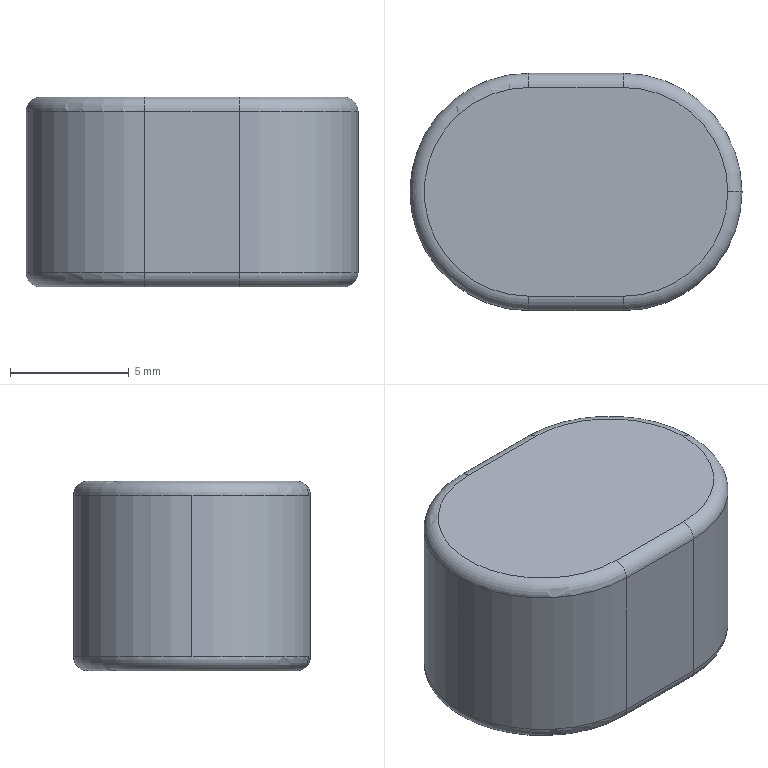Part | SolidWorks | features Extrusion 1, Fillet 1 | 1 solid | 17 faces | box 14 x 10 x 8 mm | volume 942.358 mm3 | cylinder 7 | torus 6 | plane 4 | commonest cylinder face diameters 1.2 x4 10 x3
STEP:
#1=CARTESIAN_POINT('',(6.4,0.,0.));
#2=VERTEX_POINT('',#1);
#3=CARTESIAN_POINT('',(2.,-4.4,0.));
#4=VERTEX_POINT('',#3);
#5=CARTESIAN_POINT('',(2.,0.,0.));
#6=DIRECTION('',(0.,0.,-1.));
#7=DIRECTION('',(1.,0.,0.));
#8=AXIS2_PLACEMENT_3D('',#5,#6,#7);
#9=CIRCLE('',#8,4.4);
#10=EDGE_CURVE('',#2,#4,#9,.T.);
#11=ORIENTED_EDGE('',*,*,#10,.F.);
#12=CARTESIAN_POINT('',(7.,0.,0.6));
#13=VERTEX_POINT('',#12);
#14=CARTESIAN_POINT('',(6.4,0.,0.6));
#15=DIRECTION('',(0.,-1.,0.));
#16=DIRECTION('',(0.,0.,-1.));
#17=AXIS2_PLACEMENT_3D('',#14,#15,#16);
#18=CIRCLE('',#17,0.6);
#19=EDGE_CURVE('',#2,#13,#18,.T.);
#20=ORIENTED_EDGE('',*,*,#19,.T.);
#21=CARTESIAN_POINT('',(2.,-5.,0.6));
#22=VERTEX_POINT('',#21);
#23=CARTESIAN_POINT('',(2.,0.,0.6));
#24=DIRECTION('',(0.,0.,1.));
#25=DIRECTION('',(1.,0.,0.));
#26=AXIS2_PLACEMENT_3D('',#23,#24,#25);
#27=CIRCLE('',#26,5.);
#28=EDGE_CURVE('',#22,#13,#27,.T.);
#29=ORIENTED_EDGE('',*,*,#28,.F.);
#30=CARTESIAN_POINT('',(2.,-4.4,0.6));
#31=DIRECTION('',(1.,0.,0.));
#32=DIRECTION('',(0.,0.,-1.));
#33=AXIS2_PLACEMENT_3D('',#30,#31,#32);
#34=CIRCLE('',#33,0.6);
#35=EDGE_CURVE('',#22,#4,#34,.T.);
#36=ORIENTED_EDGE('',*,*,#35,.T.);
#37=EDGE_LOOP('',(#11,#20,#29,#36));
#38=FACE_OUTER_BOUND('',#37,.T.);
#39=CARTESIAN_POINT('',(2.,0.,0.6));
#40=DIRECTION('',(0.,0.,1.));
#41=DIRECTION('',(1.,0.,0.));
#42=AXIS2_PLACEMENT_3D('',#39,#40,#41);
#43=TOROIDAL_SURFACE('',#42,4.4,0.6);
#44=ADVANCED_FACE('',(#38),#43,.T.);
#45=CARTESIAN_POINT('',(7.,0.,7.4));
#46=VERTEX_POINT('',#45);
#47=CARTESIAN_POINT('',(2.,-5.,7.4));
#48=VERTEX_POINT('',#47);
#49=CARTESIAN_POINT('',(2.,0.,7.4));
#50=DIRECTION('',(0.,0.,-1.));
#51=DIRECTION('',(1.,0.,0.));
#52=AXIS2_PLACEMENT_3D('',#49,#50,#51);
#53=CIRCLE('',#52,5.);
#54=EDGE_CURVE('',#46,#48,#53,.T.);
#55=ORIENTED_EDGE('',*,*,#54,.F.);
#56=CARTESIAN_POINT('',(6.4,0.,8.));
#57=VERTEX_POINT('',#56);
#58=CARTESIAN_POINT('',(6.4,0.,7.4));
#59=DIRECTION('',(0.,-1.,0.));
#60=DIRECTION('',(0.,0.,-1.));
#61=AXIS2_PLACEMENT_3D('',#58,#59,#60);
#62=CIRCLE('',#61,0.6);
#63=EDGE_CURVE('',#46,#57,#62,.T.);
#64=ORIENTED_EDGE('',*,*,#63,.T.);
#65=CARTESIAN_POINT('',(2.,-4.4,8.));
#66=VERTEX_POINT('',#65);
#67=CARTESIAN_POINT('',(2.,0.,8.));
#68=DIRECTION('',(0.,0.,1.));
#69=DIRECTION('',(1.,0.,0.));
#70=AXIS2_PLACEMENT_3D('',#67,#68,#69);
#71=CIRCLE('',#70,4.4);
#72=EDGE_CURVE('',#66,#57,#71,.T.);
#73=ORIENTED_EDGE('',*,*,#72,.F.);
#74=CARTESIAN_POINT('',(2.,-4.4,7.4));
#75=DIRECTION('',(1.,0.,0.));
#76=DIRECTION('',(0.,0.,-1.));
#77=AXIS2_PLACEMENT_3D('',#74,#75,#76);
#78=CIRCLE('',#77,0.6);
#79=EDGE_CURVE('',#66,#48,#78,.T.);
#80=ORIENTED_EDGE('',*,*,#79,.T.);
#81=EDGE_LOOP('',(#55,#64,#73,#80));
#82=FACE_OUTER_BOUND('',#81,.T.);
#83=CARTESIAN_POINT('',(2.,0.,7.4));
#84=DIRECTION('',(0.,0.,1.));
#85=DIRECTION('',(1.,0.,0.));
#86=AXIS2_PLACEMENT_3D('',#83,#84,#85);
#87=TOROIDAL_SURFACE('',#86,4.4,0.6);
#88=ADVANCED_FACE('',(#82),#87,.T.);
#89=CARTESIAN_POINT('',(-2.,-5.,7.4));
#90=VERTEX_POINT('',#89);
#91=CARTESIAN_POINT('',(-7.,0.,7.4));
#92=VERTEX_POINT('',#91);
#93=CARTESIAN_POINT('',(-2.,0.,7.4));
#94=DIRECTION('',(0.,0.,-1.));
#95=DIRECTION('',(1.,0.,0.));
#96=AXIS2_PLACEMENT_3D('',#93,#94,#95);
#97=CIRCLE('',#96,5.);
#98=EDGE_CURVE('',#90,#92,#97,.T.);
#99=ORIENTED_EDGE('',*,*,#98,.T.);
#100=CARTESIAN_POINT('',(-7.,0.,0.6));
#101=VERTEX_POINT('',#100);
#102=CARTESIAN_POINT('',(-7.,0.,8.));
#103=DIRECTION('',(0.,0.,-1.));
#104=VECTOR('',#103,1000.);
#105=LINE('',#102,#104);
#106=EDGE_CURVE('',#92,#101,#105,.T.);
#107=ORIENTED_EDGE('',*,*,#106,.T.);
#108=CARTESIAN_POINT('',(-2.,-5.,0.6));
#109=VERTEX_POINT('',#108);
#110=CARTESIAN_POINT('',(-2.,0.,0.6));
#111=DIRECTION('',(0.,0.,1.));
#112=DIRECTION('',(1.,0.,0.));
#113=AXIS2_PLACEMENT_3D('',#110,#111,#112);
#114=CIRCLE('',#113,5.);
#115=EDGE_CURVE('',#101,#109,#114,.T.);
#116=ORIENTED_EDGE('',*,*,#115,.T.);
#117=CARTESIAN_POINT('',(-2.,-5.,8.));
#118=DIRECTION('',(0.,0.,-1.));
#119=VECTOR('',#118,1000.);
#120=LINE('',#117,#119);
#121=EDGE_CURVE('',#90,#109,#120,.T.);
#122=ORIENTED_EDGE('',*,*,#121,.F.);
#123=EDGE_LOOP('',(#99,#107,#116,#122));
#124=FACE_OUTER_BOUND('',#123,.T.);
#125=CARTESIAN_POINT('',(-2.,0.,8.));
#126=DIRECTION('',(0.,0.,-1.));
#127=DIRECTION('',(-1.,0.,0.));
#128=AXIS2_PLACEMENT_3D('',#125,#126,#127);
#129=CYLINDRICAL_SURFACE('',#128,5.);
#130=ADVANCED_FACE('',(#124),#129,.T.);
#131=ORIENTED_EDGE('',*,*,#106,.F.);
#132=CARTESIAN_POINT('',(-2.,5.,7.4));
#133=VERTEX_POINT('',#132);
#134=CARTESIAN_POINT('',(-2.,0.,7.4));
#135=DIRECTION('',(0.,0.,-1.));
#136=DIRECTION('',(1.,0.,0.));
#137=AXIS2_PLACEMENT_3D('',#134,#135,#136);
#138=CIRCLE('',#137,5.);
#139=EDGE_CURVE('',#92,#133,#138,.T.);
#140=ORIENTED_EDGE('',*,*,#139,.T.);
#141=CARTESIAN_POINT('',(-2.,5.,0.6));
#142=VERTEX_POINT('',#141);
#143=CARTESIAN_POINT('',(-2.,5.,8.));
#144=DIRECTION('',(0.,0.,-1.));
#145=VECTOR('',#144,1000.);
#146=LINE('',#143,#145);
#147=EDGE_CURVE('',#133,#142,#146,.T.);
#148=ORIENTED_EDGE('',*,*,#147,.T.);
#149=CARTESIAN_POINT('',(-2.,0.,0.6));
#150=DIRECTION('',(0.,0.,1.));
#151=DIRECTION('',(1.,0.,0.));
#152=AXIS2_PLACEMENT_3D('',#149,#150,#151);
#153=CIRCLE('',#152,5.);
#154=EDGE_CURVE('',#142,#101,#153,.T.);
#155=ORIENTED_EDGE('',*,*,#154,.T.);
#156=EDGE_LOOP('',(#131,#140,#148,#155));
#157=FACE_OUTER_BOUND('',#156,.T.);
#158=CARTESIAN_POINT('',(-2.,0.,8.));
#159=DIRECTION('',(0.,0.,-1.));
#160=DIRECTION('',(-1.,0.,0.));
#161=AXIS2_PLACEMENT_3D('',#158,#159,#160);
#162=CYLINDRICAL_SURFACE('',#161,5.);
#163=ADVANCED_FACE('',(#157),#162,.T.);
#164=CARTESIAN_POINT('',(2.,-5.,8.));
#165=DIRECTION('',(0.,0.,-1.));
#166=VECTOR('',#165,1000.);
#167=LINE('',#164,#166);
#168=EDGE_CURVE('',#48,#22,#167,.T.);
#169=ORIENTED_EDGE('',*,*,#168,.F.);
#170=CARTESIAN_POINT('',(-2.,-5.,7.4));
#171=DIRECTION('',(-1.,0.,0.));
#172=VECTOR('',#171,1000.);
#173=LINE('',#170,#172);
#174=EDGE_CURVE('',#48,#90,#173,.T.);
#175=ORIENTED_EDGE('',*,*,#174,.T.);
#176=ORIENTED_EDGE('',*,*,#121,.T.);
#177=CARTESIAN_POINT('',(-2.,-5.,0.6));
#178=DIRECTION('',(1.,0.,0.));
#179=VECTOR('',#178,1000.);
#180=LINE('',#177,#179);
#181=EDGE_CURVE('',#109,#22,#180,.T.);
#182=ORIENTED_EDGE('',*,*,#181,.T.);
#183=EDGE_LOOP('',(#169,#175,#176,#182));
#184=FACE_OUTER_BOUND('',#183,.T.);
#185=CARTESIAN_POINT('',(-2.,-5.,8.));
#186=DIRECTION('',(0.,1.,0.));
#187=DIRECTION('',(-1.,0.,0.));
#188=AXIS2_PLACEMENT_3D('',#185,#186,#187);
#189=PLANE('',#188);
#190=ADVANCED_FACE('',(#184),#189,.F.);
#191=CARTESIAN_POINT('',(2.,5.,7.4));
#192=VERTEX_POINT('',#191);
#193=CARTESIAN_POINT('',(2.,5.,0.6));
#194=VERTEX_POINT('',#193);
#195=CARTESIAN_POINT('',(2.,5.,8.));
#196=DIRECTION('',(0.,0.,-1.));
#197=VECTOR('',#196,1000.);
#198=LINE('',#195,#197);
#199=EDGE_CURVE('',#192,#194,#198,.T.);
#200=ORIENTED_EDGE('',*,*,#199,.F.);
#201=CARTESIAN_POINT('',(2.,0.,7.4));
#202=DIRECTION('',(0.,0.,-1.));
#203=DIRECTION('',(1.,0.,0.));
#204=AXIS2_PLACEMENT_3D('',#201,#202,#203);
#205=CIRCLE('',#204,5.);
#206=EDGE_CURVE('',#192,#46,#205,.T.);
#207=ORIENTED_EDGE('',*,*,#206,.T.);
#208=ORIENTED_EDGE('',*,*,#54,.T.);
#209=ORIENTED_EDGE('',*,*,#168,.T.);
#210=ORIENTED_EDGE('',*,*,#28,.T.);
#211=CARTESIAN_POINT('',(2.,0.,0.6));
#212=DIRECTION('',(0.,0.,1.));
#213=DIRECTION('',(1.,0.,0.));
#214=AXIS2_PLACEMENT_3D('',#211,#212,#213);
#215=CIRCLE('',#214,5.);
#216=EDGE_CURVE('',#13,#194,#215,.T.);
#217=ORIENTED_EDGE('',*,*,#216,.T.);
#218=EDGE_LOOP('',(#200,#207,#208,#209,#210,#217));
#219=FACE_OUTER_BOUND('',#218,.T.);
#220=CARTESIAN_POINT('',(2.,0.,8.));
#221=DIRECTION('',(0.,0.,-1.));
#222=DIRECTION('',(-1.,0.,0.));
#223=AXIS2_PLACEMENT_3D('',#220,#221,#222);
#224=CYLINDRICAL_SURFACE('',#223,5.);
#225=ADVANCED_FACE('',(#219),#224,.T.);
#226=ORIENTED_EDGE('',*,*,#147,.F.);
#227=CARTESIAN_POINT('',(2.,5.,7.4));
#228=DIRECTION('',(1.,0.,0.));
#229=VECTOR('',#228,1000.);
#230=LINE('',#227,#229);
#231=EDGE_CURVE('',#133,#192,#230,.T.);
#232=ORIENTED_EDGE('',*,*,#231,.T.);
#233=ORIENTED_EDGE('',*,*,#199,.T.);
#234=CARTESIAN_POINT('',(-2.,5.,0.6));
#235=DIRECTION('',(-1.,0.,0.));
#236=VECTOR('',#235,1000.);
#237=LINE('',#234,#236);
#238=EDGE_CURVE('',#194,#142,#237,.T.);
#239=ORIENTED_EDGE('',*,*,#238,.T.);
#240=EDGE_LOOP('',(#226,#232,#233,#239));
#241=FACE_OUTER_BOUND('',#240,.T.);
#242=CARTESIAN_POINT('',(-2.,5.,8.));
#243=DIRECTION('',(0.,-1.,0.));
#244=DIRECTION('',(1.,0.,0.));
#245=AXIS2_PLACEMENT_3D('',#242,#243,#244);
#246=PLANE('',#245);
#247=ADVANCED_FACE('',(#241),#246,.F.);
#248=CARTESIAN_POINT('',(-2.,-4.4,8.));
#249=VERTEX_POINT('',#248);
#250=CARTESIAN_POINT('',(2.,-4.4,8.));
#251=DIRECTION('',(1.,0.,0.));
#252=VECTOR('',#251,1000.);
#253=LINE('',#250,#252);
#254=EDGE_CURVE('',#249,#66,#253,.T.);
#255=ORIENTED_EDGE('',*,*,#254,.T.);
#256=ORIENTED_EDGE('',*,*,#72,.T.);
#257=CARTESIAN_POINT('',(2.,4.4,8.));
#258=VERTEX_POINT('',#257);
#259=CARTESIAN_POINT('',(2.,0.,8.));
#260=DIRECTION('',(0.,0.,1.));
#261=DIRECTION('',(1.,0.,0.));
#262=AXIS2_PLACEMENT_3D('',#259,#260,#261);
#263=CIRCLE('',#262,4.4);
#264=EDGE_CURVE('',#57,#258,#263,.T.);
#265=ORIENTED_EDGE('',*,*,#264,.T.);
#266=CARTESIAN_POINT('',(-2.,4.4,8.));
#267=VERTEX_POINT('',#266);
#268=CARTESIAN_POINT('',(-2.,4.4,8.));
#269=DIRECTION('',(-1.,0.,0.));
#270=VECTOR('',#269,1000.);
#271=LINE('',#268,#270);
#272=EDGE_CURVE('',#258,#267,#271,.T.);
#273=ORIENTED_EDGE('',*,*,#272,.T.);
#274=CARTESIAN_POINT('',(-2.,0.,8.));
#275=DIRECTION('',(0.,0.,1.));
#276=DIRECTION('',(1.,0.,0.));
#277=AXIS2_PLACEMENT_3D('',#274,#275,#276);
#278=CIRCLE('',#277,4.4);
#279=EDGE_CURVE('',#267,#249,#278,.T.);
#280=ORIENTED_EDGE('',*,*,#279,.T.);
#281=EDGE_LOOP('',(#255,#256,#265,#273,#280));
#282=FACE_OUTER_BOUND('',#281,.T.);
#283=CARTESIAN_POINT('',(-2.,0.,8.));
#284=DIRECTION('',(0.,0.,1.));
#285=DIRECTION('',(1.,0.,0.));
#286=AXIS2_PLACEMENT_3D('',#283,#284,#285);
#287=PLANE('',#286);
#288=ADVANCED_FACE('',(#282),#287,.T.);
#289=CARTESIAN_POINT('',(-2.,4.4,0.));
#290=VERTEX_POINT('',#289);
#291=CARTESIAN_POINT('',(2.,4.4,0.));
#292=VERTEX_POINT('',#291);
#293=CARTESIAN_POINT('',(-2.,4.4,0.));
#294=DIRECTION('',(1.,0.,0.));
#295=VECTOR('',#294,1000.);
#296=LINE('',#293,#295);
#297=EDGE_CURVE('',#290,#292,#296,.T.);
#298=ORIENTED_EDGE('',*,*,#297,.T.);
#299=CARTESIAN_POINT('',(2.,0.,0.));
#300=DIRECTION('',(0.,0.,-1.));
#301=DIRECTION('',(1.,0.,0.));
#302=AXIS2_PLACEMENT_3D('',#299,#300,#301);
#303=CIRCLE('',#302,4.4);
#304=EDGE_CURVE('',#292,#2,#303,.T.);
#305=ORIENTED_EDGE('',*,*,#304,.T.);
#306=ORIENTED_EDGE('',*,*,#10,.T.);
#307=CARTESIAN_POINT('',(-2.,-4.4,0.));
#308=VERTEX_POINT('',#307);
#309=CARTESIAN_POINT('',(-2.,-4.4,0.));
#310=DIRECTION('',(-1.,0.,0.));
#311=VECTOR('',#310,1000.);
#312=LINE('',#309,#311);
#313=EDGE_CURVE('',#4,#308,#312,.T.);
#314=ORIENTED_EDGE('',*,*,#313,.T.);
#315=CARTESIAN_POINT('',(-2.,0.,0.));
#316=DIRECTION('',(0.,0.,-1.));
#317=DIRECTION('',(1.,0.,0.));
#318=AXIS2_PLACEMENT_3D('',#315,#316,#317);
#319=CIRCLE('',#318,4.4);
#320=EDGE_CURVE('',#308,#290,#319,.T.);
#321=ORIENTED_EDGE('',*,*,#320,.T.);
#322=EDGE_LOOP('',(#298,#305,#306,#314,#321));
#323=FACE_OUTER_BOUND('',#322,.T.);
#324=CARTESIAN_POINT('',(-2.,0.,0.));
#325=DIRECTION('',(0.,0.,1.));
#326=DIRECTION('',(1.,0.,0.));
#327=AXIS2_PLACEMENT_3D('',#324,#325,#326);
#328=PLANE('',#327);
#329=ADVANCED_FACE('',(#323),#328,.F.);
#330=CARTESIAN_POINT('',(-2.,4.4,7.4));
#331=DIRECTION('',(1.,0.,0.));
#332=DIRECTION('',(0.,0.,-1.));
#333=AXIS2_PLACEMENT_3D('',#330,#331,#332);
#334=CIRCLE('',#333,0.6);
#335=EDGE_CURVE('',#133,#267,#334,.T.);
#336=ORIENTED_EDGE('',*,*,#335,.F.);
#337=ORIENTED_EDGE('',*,*,#139,.F.);
#338=ORIENTED_EDGE('',*,*,#98,.F.);
#339=CARTESIAN_POINT('',(-2.,-4.4,7.4));
#340=DIRECTION('',(1.,0.,0.));
#341=DIRECTION('',(0.,0.,-1.));
#342=AXIS2_PLACEMENT_3D('',#339,#340,#341);
#343=CIRCLE('',#342,0.6);
#344=EDGE_CURVE('',#249,#90,#343,.T.);
#345=ORIENTED_EDGE('',*,*,#344,.F.);
#346=ORIENTED_EDGE('',*,*,#279,.F.);
#347=EDGE_LOOP('',(#336,#337,#338,#345,#346));
#348=FACE_OUTER_BOUND('',#347,.T.);
#349=CARTESIAN_POINT('',(-2.,0.,7.4));
#350=DIRECTION('',(0.,0.,1.));
#351=DIRECTION('',(1.,0.,0.));
#352=AXIS2_PLACEMENT_3D('',#349,#350,#351);
#353=TOROIDAL_SURFACE('',#352,4.4,0.6);
#354=ADVANCED_FACE('',(#348),#353,.T.);
#355=ORIENTED_EDGE('',*,*,#344,.T.);
#356=ORIENTED_EDGE('',*,*,#174,.F.);
#357=ORIENTED_EDGE('',*,*,#79,.F.);
#358=ORIENTED_EDGE('',*,*,#254,.F.);
#359=EDGE_LOOP('',(#355,#356,#357,#358));
#360=FACE_OUTER_BOUND('',#359,.T.);
#361=CARTESIAN_POINT('',(-2.,-4.4,7.4));
#362=DIRECTION('',(-1.,0.,0.));
#363=DIRECTION('',(0.,-1.,0.));
#364=AXIS2_PLACEMENT_3D('',#361,#362,#363);
#365=CYLINDRICAL_SURFACE('',#364,0.6);
#366=ADVANCED_FACE('',(#360),#365,.T.);
#367=ORIENTED_EDGE('',*,*,#335,.T.);
#368=ORIENTED_EDGE('',*,*,#272,.F.);
#369=CARTESIAN_POINT('',(2.,4.4,7.4));
#370=DIRECTION('',(1.,0.,0.));
#371=DIRECTION('',(0.,0.,-1.));
#372=AXIS2_PLACEMENT_3D('',#369,#370,#371);
#373=CIRCLE('',#372,0.6);
#374=EDGE_CURVE('',#192,#258,#373,.T.);
#375=ORIENTED_EDGE('',*,*,#374,.F.);
#376=ORIENTED_EDGE('',*,*,#231,.F.);
#377=EDGE_LOOP('',(#367,#368,#375,#376));
#378=FACE_OUTER_BOUND('',#377,.T.);
#379=CARTESIAN_POINT('',(-2.,4.4,7.4));
#380=DIRECTION('',(1.,0.,0.));
#381=DIRECTION('',(0.,1.,0.));
#382=AXIS2_PLACEMENT_3D('',#379,#380,#381);
#383=CYLINDRICAL_SURFACE('',#382,0.6);
#384=ADVANCED_FACE('',(#378),#383,.T.);
#385=ORIENTED_EDGE('',*,*,#63,.F.);
#386=ORIENTED_EDGE('',*,*,#206,.F.);
#387=ORIENTED_EDGE('',*,*,#374,.T.);
#388=ORIENTED_EDGE('',*,*,#264,.F.);
#389=EDGE_LOOP('',(#385,#386,#387,#388));
#390=FACE_OUTER_BOUND('',#389,.T.);
#391=CARTESIAN_POINT('',(2.,0.,7.4));
#392=DIRECTION('',(0.,0.,1.));
#393=DIRECTION('',(1.,0.,0.));
#394=AXIS2_PLACEMENT_3D('',#391,#392,#393);
#395=TOROIDAL_SURFACE('',#394,4.4,0.6);
#396=ADVANCED_FACE('',(#390),#395,.T.);
#397=CARTESIAN_POINT('',(-2.,4.4,0.6));
#398=DIRECTION('',(1.,0.,0.));
#399=DIRECTION('',(0.,0.,-1.));
#400=AXIS2_PLACEMENT_3D('',#397,#398,#399);
#401=CIRCLE('',#400,0.6);
#402=EDGE_CURVE('',#290,#142,#401,.T.);
#403=ORIENTED_EDGE('',*,*,#402,.F.);
#404=ORIENTED_EDGE('',*,*,#320,.F.);
#405=CARTESIAN_POINT('',(-2.,-4.4,0.6));
#406=DIRECTION('',(1.,0.,0.));
#407=DIRECTION('',(0.,0.,-1.));
#408=AXIS2_PLACEMENT_3D('',#405,#406,#407);
#409=CIRCLE('',#408,0.6);
#410=EDGE_CURVE('',#109,#308,#409,.T.);
#411=ORIENTED_EDGE('',*,*,#410,.F.);
#412=ORIENTED_EDGE('',*,*,#115,.F.);
#413=ORIENTED_EDGE('',*,*,#154,.F.);
#414=EDGE_LOOP('',(#403,#404,#411,#412,#413));
#415=FACE_OUTER_BOUND('',#414,.T.);
#416=CARTESIAN_POINT('',(-2.,0.,0.6));
#417=DIRECTION('',(0.,0.,1.));
#418=DIRECTION('',(1.,0.,0.));
#419=AXIS2_PLACEMENT_3D('',#416,#417,#418);
#420=TOROIDAL_SURFACE('',#419,4.4,0.6);
#421=ADVANCED_FACE('',(#415),#420,.T.);
#422=ORIENTED_EDGE('',*,*,#410,.T.);
#423=ORIENTED_EDGE('',*,*,#313,.F.);
#424=ORIENTED_EDGE('',*,*,#35,.F.);
#425=ORIENTED_EDGE('',*,*,#181,.F.);
#426=EDGE_LOOP('',(#422,#423,#424,#425));
#427=FACE_OUTER_BOUND('',#426,.T.);
#428=CARTESIAN_POINT('',(-2.,-4.4,0.6));
#429=DIRECTION('',(1.,0.,0.));
#430=DIRECTION('',(0.,1.,0.));
#431=AXIS2_PLACEMENT_3D('',#428,#429,#430);
#432=CYLINDRICAL_SURFACE('',#431,0.6);
#433=ADVANCED_FACE('',(#427),#432,.T.);
#434=ORIENTED_EDGE('',*,*,#402,.T.);
#435=ORIENTED_EDGE('',*,*,#238,.F.);
#436=CARTESIAN_POINT('',(2.,4.4,0.6));
#437=DIRECTION('',(1.,0.,0.));
#438=DIRECTION('',(0.,0.,-1.));
#439=AXIS2_PLACEMENT_3D('',#436,#437,#438);
#440=CIRCLE('',#439,0.6);
#441=EDGE_CURVE('',#292,#194,#440,.T.);
#442=ORIENTED_EDGE('',*,*,#441,.F.);
#443=ORIENTED_EDGE('',*,*,#297,.F.);
#444=EDGE_LOOP('',(#434,#435,#442,#443));
#445=FACE_OUTER_BOUND('',#444,.T.);
#446=CARTESIAN_POINT('',(-2.,4.4,0.6));
#447=DIRECTION('',(-1.,0.,0.));
#448=DIRECTION('',(0.,-1.,0.));
#449=AXIS2_PLACEMENT_3D('',#446,#447,#448);
#450=CYLINDRICAL_SURFACE('',#449,0.6);
#451=ADVANCED_FACE('',(#445),#450,.T.);
#452=ORIENTED_EDGE('',*,*,#19,.F.);
#453=ORIENTED_EDGE('',*,*,#304,.F.);
#454=ORIENTED_EDGE('',*,*,#441,.T.);
#455=ORIENTED_EDGE('',*,*,#216,.F.);
#456=EDGE_LOOP('',(#452,#453,#454,#455));
#457=FACE_OUTER_BOUND('',#456,.T.);
#458=CARTESIAN_POINT('',(2.,0.,0.6));
#459=DIRECTION('',(0.,0.,1.));
#460=DIRECTION('',(1.,0.,0.));
#461=AXIS2_PLACEMENT_3D('',#458,#459,#460);
#462=TOROIDAL_SURFACE('',#461,4.4,0.6);
#463=ADVANCED_FACE('',(#457),#462,.T.);
#464=CLOSED_SHELL('',(#44,#88,#130,#163,#190,#225,#247,#288,#329,#354,#366,#384,#396,#421,#433,#451,#463));
#465=MANIFOLD_SOLID_BREP('',#464);
#466=CARTESIAN_POINT('',(0.,0.,0.));
#467=DIRECTION('',(0.,0.,1.));
#468=DIRECTION('',(1.,0.,0.));
#469=AXIS2_PLACEMENT_3D('',#466,#467,#468);
#470=(LENGTH_UNIT()NAMED_UNIT(*)SI_UNIT(.MILLI.,.METRE.));
#471=UNCERTAINTY_MEASURE_WITH_UNIT(LENGTH_MEASURE(0.00001),#470,'','');
#472=(NAMED_UNIT(*)PLANE_ANGLE_UNIT()SI_UNIT($,.RADIAN.));
#473=(NAMED_UNIT(*)SI_UNIT($,.STERADIAN.)SOLID_ANGLE_UNIT());
#474=(GEOMETRIC_REPRESENTATION_CONTEXT(3)GLOBAL_UNCERTAINTY_ASSIGNED_CONTEXT((#471))GLOBAL_UNIT_ASSIGNED_CONTEXT((#470,#472,#473))REPRESENTATION_CONTEXT('',''));
#475=ADVANCED_BREP_SHAPE_REPRESENTATION('',(#465,#469),#474);